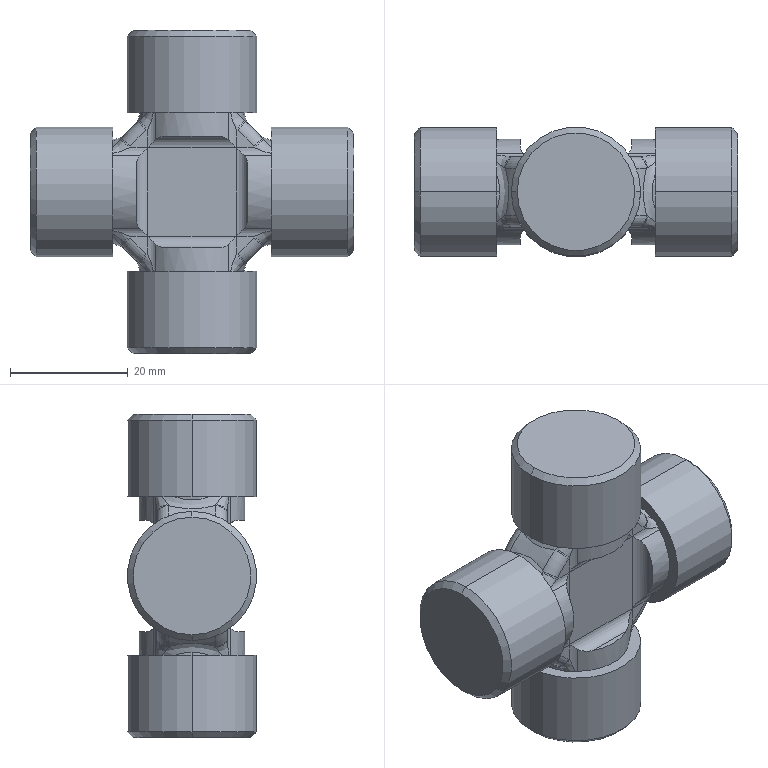Part | STEP file | CARDAN_COUPLING1V11 | 1 solid | 138 faces | box 55 x 22 x 55 mm | volume 30051 mm3 | cylinder 56 | spline 40 | plane 26 | cone 8 | torus 8 | commonest cylinder face diameters 4 x24 18 x20 22 x8 30 x4